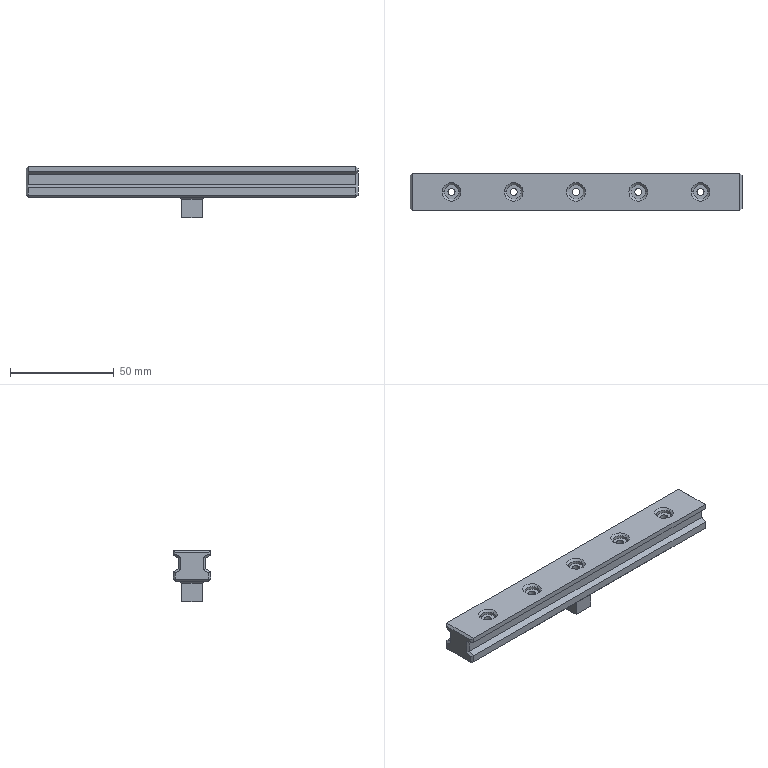Part | SolidWorks | features Chamfer 3, ICE 2, 3DProfileFeature 1, Extrusion 1, HoleWzd 1, LPattern 1, MirrorPattern 1 | 1 solid | 88 faces | box 160 x 18 x 25 mm | volume 37654 mm3 | plane 58 | cylinder 20 | cone 10 | commonest cylinder face diameters 3.4 x10 7 x10